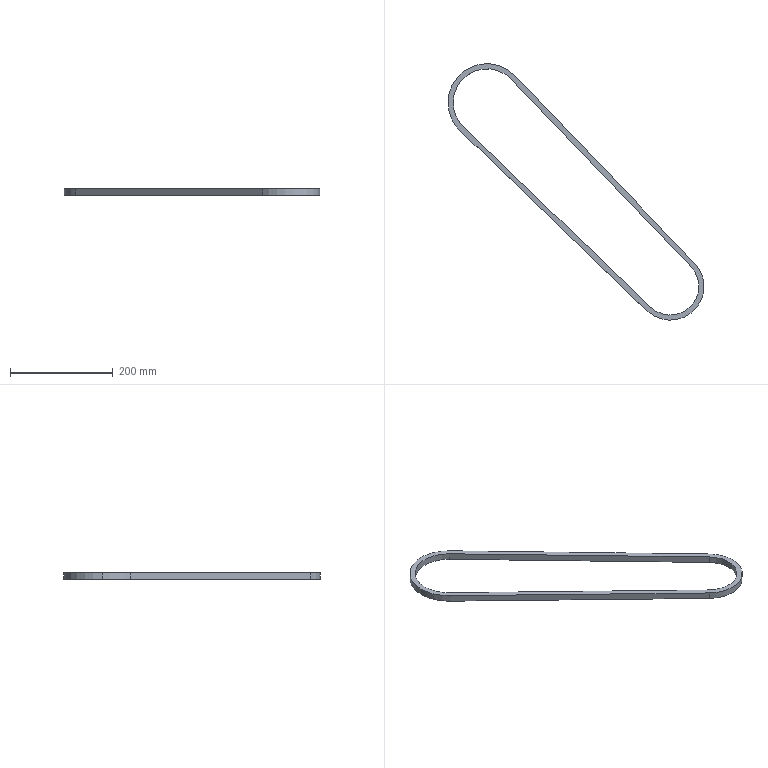Part | STEP file | Pasek_klinowy3V11 | 1 solid | 12 faces | box 497.285 x 498.317 x 13 mm | volume 184721 mm3 | cylinder 6 | plane 6 | commonest cylinder face diameters 131 x3 151 x2 111 x1
STEP:
#1=CARTESIAN_POINT('',(0.,0.,0.));
#2=DIRECTION('',(0.,0.,1.));
#3=DIRECTION('',(1.,0.,0.));
#4=AXIS2_PLACEMENT_3D('',#1,#2,#3);
#5=CARTESIAN_POINT('',(226.295,-74.498,13.));
#6=VERTEX_POINT('',#5);
#7=CARTESIAN_POINT('',(226.295,-74.498,0.));
#8=VERTEX_POINT('',#7);
#9=CARTESIAN_POINT('',(226.295,-74.498,13.));
#10=DIRECTION('',(0.,0.,-1.));
#11=VECTOR('',#10,1.);
#12=LINE('',#9,#11);
#13=CARTESIAN_POINT('',(179.005,-119.818,13.));
#14=DIRECTION('',(0.,0.,-1.));
#15=DIRECTION('',(-1.,0.,0.));
#16=AXIS2_PLACEMENT_3D('',#13,#14,#15);
#17=CYLINDRICAL_SURFACE('',#16,65.5);
#18=CARTESIAN_POINT('',(2.377,0.));
#19=DIRECTION('',(0.,1.));
#20=VECTOR('',#19,1.);
#21=LINE('',#18,#20);
#22=(GEOMETRIC_REPRESENTATION_CONTEXT(2)PARAMETRIC_REPRESENTATION_CONTEXT()REPRESENTATION_CONTEXT('',''));
#23=DEFINITIONAL_REPRESENTATION('',(#21),#22);
#24=PCURVE('',#17,#23);
#25=CARTESIAN_POINT('',(226.295,-74.498,13.));
#26=DIRECTION('',(-0.722,-0.6919,0.));
#27=DIRECTION('',(0.6919,-0.722,0.));
#28=AXIS2_PLACEMENT_3D('',#25,#26,#27);
#29=PLANE('',#28);
#30=CARTESIAN_POINT('',(0.,0.));
#31=DIRECTION('',(0.,-1.));
#32=VECTOR('',#31,1.);
#33=LINE('',#30,#32);
#34=(GEOMETRIC_REPRESENTATION_CONTEXT(2)PARAMETRIC_REPRESENTATION_CONTEXT()REPRESENTATION_CONTEXT('',''));
#35=DEFINITIONAL_REPRESENTATION('',(#33),#34);
#36=PCURVE('',#29,#35);
#37=SURFACE_CURVE('',#12,(#24,#36),.PCURVE_S1.);
#38=EDGE_CURVE('',#6,#8,#37,.T.);
#39=ORIENTED_EDGE('',*,*,#38,.T.);
#40=CARTESIAN_POINT('',(113.505,-119.818,0.));
#41=VERTEX_POINT('',#40);
#42=CARTESIAN_POINT('',(179.005,-119.818,0.));
#43=DIRECTION('',(0.,0.,1.));
#44=DIRECTION('',(1.,0.,0.));
#45=AXIS2_PLACEMENT_3D('',#42,#43,#44);
#46=CIRCLE('',#45,65.5);
#47=CARTESIAN_POINT('',(3.142,13.));
#48=DIRECTION('',(-1.,0.));
#49=VECTOR('',#48,1.);
#50=LINE('',#47,#49);
#51=(GEOMETRIC_REPRESENTATION_CONTEXT(2)PARAMETRIC_REPRESENTATION_CONTEXT()REPRESENTATION_CONTEXT('',''));
#52=DEFINITIONAL_REPRESENTATION('',(#50),#51);
#53=PCURVE('',#17,#52);
#54=CARTESIAN_POINT('',(179.005,-119.818,0.));
#55=DIRECTION('',(0.,0.,1.));
#56=DIRECTION('',(1.,0.,0.));
#57=AXIS2_PLACEMENT_3D('',#54,#55,#56);
#58=PLANE('',#57);
#59=CARTESIAN_POINT('',(0.,0.));
#60=DIRECTION('',(1.,0.));
#61=AXIS2_PLACEMENT_2D('',#59,#60);
#62=CIRCLE('',#61,65.5);
#63=(GEOMETRIC_REPRESENTATION_CONTEXT(2)PARAMETRIC_REPRESENTATION_CONTEXT()REPRESENTATION_CONTEXT('',''));
#64=DEFINITIONAL_REPRESENTATION('',(#62),#63);
#65=PCURVE('',#58,#64);
#66=SURFACE_CURVE('',#46,(#53,#65),.PCURVE_S1.);
#67=EDGE_CURVE('',#8,#41,#66,.T.);
#68=ORIENTED_EDGE('',*,*,#67,.T.);
#69=CARTESIAN_POINT('',(113.505,-119.818,13.));
#70=VERTEX_POINT('',#69);
#71=CARTESIAN_POINT('',(113.505,-119.818,13.));
#72=DIRECTION('',(0.,0.,-1.));
#73=VECTOR('',#72,1.);
#74=LINE('',#71,#73);
#75=CARTESIAN_POINT('',(0.,0.));
#76=DIRECTION('',(0.,1.));
#77=VECTOR('',#76,1.);
#78=LINE('',#75,#77);
#79=(GEOMETRIC_REPRESENTATION_CONTEXT(2)PARAMETRIC_REPRESENTATION_CONTEXT()REPRESENTATION_CONTEXT('',''));
#80=DEFINITIONAL_REPRESENTATION('',(#78),#79);
#81=PCURVE('',#17,#80);
#82=CARTESIAN_POINT('',(179.005,-119.818,13.));
#83=DIRECTION('',(0.,0.,-1.));
#84=DIRECTION('',(-1.,0.,0.));
#85=AXIS2_PLACEMENT_3D('',#82,#83,#84);
#86=CYLINDRICAL_SURFACE('',#85,65.5);
#87=CARTESIAN_POINT('',(6.283,0.));
#88=DIRECTION('',(0.,1.));
#89=VECTOR('',#88,1.);
#90=LINE('',#87,#89);
#91=(GEOMETRIC_REPRESENTATION_CONTEXT(2)PARAMETRIC_REPRESENTATION_CONTEXT()REPRESENTATION_CONTEXT('',''));
#92=DEFINITIONAL_REPRESENTATION('',(#90),#91);
#93=PCURVE('',#86,#92);
#94=SURFACE_CURVE('',#74,(#81,#93),.PCURVE_S1.);
#95=EDGE_CURVE('',#70,#41,#94,.T.);
#96=ORIENTED_EDGE('',*,*,#95,.F.);
#97=CARTESIAN_POINT('',(179.005,-119.818,13.));
#98=DIRECTION('',(0.,0.,1.));
#99=DIRECTION('',(1.,0.,0.));
#100=AXIS2_PLACEMENT_3D('',#97,#98,#99);
#101=CIRCLE('',#100,65.5);
#102=CARTESIAN_POINT('',(3.142,0.));
#103=DIRECTION('',(-1.,0.));
#104=VECTOR('',#103,1.);
#105=LINE('',#102,#104);
#106=(GEOMETRIC_REPRESENTATION_CONTEXT(2)PARAMETRIC_REPRESENTATION_CONTEXT()REPRESENTATION_CONTEXT('',''));
#107=DEFINITIONAL_REPRESENTATION('',(#105),#106);
#108=PCURVE('',#17,#107);
#109=CARTESIAN_POINT('',(179.005,-119.818,13.));
#110=DIRECTION('',(0.,0.,1.));
#111=DIRECTION('',(1.,0.,0.));
#112=AXIS2_PLACEMENT_3D('',#109,#110,#111);
#113=PLANE('',#112);
#114=CARTESIAN_POINT('',(0.,0.));
#115=DIRECTION('',(1.,0.));
#116=AXIS2_PLACEMENT_2D('',#114,#115);
#117=CIRCLE('',#116,65.5);
#118=(GEOMETRIC_REPRESENTATION_CONTEXT(2)PARAMETRIC_REPRESENTATION_CONTEXT()REPRESENTATION_CONTEXT('',''));
#119=DEFINITIONAL_REPRESENTATION('',(#117),#118);
#120=PCURVE('',#113,#119);
#121=SURFACE_CURVE('',#101,(#108,#120),.PCURVE_S1.);
#122=EDGE_CURVE('',#6,#70,#121,.T.);
#123=ORIENTED_EDGE('',*,*,#122,.F.);
#124=EDGE_LOOP('',(#39,#68,#96,#123));
#125=FACE_BOUND('',#124,.F.);
#126=ADVANCED_FACE('',(#125),#17,.F.);
#127=CARTESIAN_POINT('',(103.505,-119.818,13.));
#128=VERTEX_POINT('',#127);
#129=CARTESIAN_POINT('',(126.608,-174.177,13.));
#130=VERTEX_POINT('',#129);
#131=CARTESIAN_POINT('',(179.005,-119.818,13.));
#132=DIRECTION('',(0.,0.,1.));
#133=DIRECTION('',(1.,0.,0.));
#134=AXIS2_PLACEMENT_3D('',#131,#132,#133);
#135=CIRCLE('',#134,75.5);
#136=CARTESIAN_POINT('',(179.005,-119.818,13.));
#137=DIRECTION('',(0.,0.,-1.));
#138=DIRECTION('',(-1.,0.,0.));
#139=AXIS2_PLACEMENT_3D('',#136,#137,#138);
#140=CYLINDRICAL_SURFACE('',#139,75.5);
#141=CARTESIAN_POINT('',(9.425,0.));
#142=DIRECTION('',(-1.,0.));
#143=VECTOR('',#142,1.);
#144=LINE('',#141,#143);
#145=(GEOMETRIC_REPRESENTATION_CONTEXT(2)PARAMETRIC_REPRESENTATION_CONTEXT()REPRESENTATION_CONTEXT('',''));
#146=DEFINITIONAL_REPRESENTATION('',(#144),#145);
#147=PCURVE('',#140,#146);
#148=CARTESIAN_POINT('',(0.,0.));
#149=DIRECTION('',(1.,0.));
#150=AXIS2_PLACEMENT_2D('',#148,#149);
#151=CIRCLE('',#150,75.5);
#152=(GEOMETRIC_REPRESENTATION_CONTEXT(2)PARAMETRIC_REPRESENTATION_CONTEXT()REPRESENTATION_CONTEXT('',''));
#153=DEFINITIONAL_REPRESENTATION('',(#151),#152);
#154=PCURVE('',#113,#153);
#155=SURFACE_CURVE('',#135,(#147,#154),.PCURVE_S1.);
#156=EDGE_CURVE('',#128,#130,#155,.T.);
#157=ORIENTED_EDGE('',*,*,#156,.F.);
#158=CARTESIAN_POINT('',(103.505,-119.818,0.));
#159=VERTEX_POINT('',#158);
#160=CARTESIAN_POINT('',(103.505,-119.818,13.));
#161=DIRECTION('',(0.,0.,-1.));
#162=VECTOR('',#161,1.);
#163=LINE('',#160,#162);
#164=CARTESIAN_POINT('',(6.283,0.));
#165=DIRECTION('',(0.,1.));
#166=VECTOR('',#165,1.);
#167=LINE('',#164,#166);
#168=(GEOMETRIC_REPRESENTATION_CONTEXT(2)PARAMETRIC_REPRESENTATION_CONTEXT()REPRESENTATION_CONTEXT('',''));
#169=DEFINITIONAL_REPRESENTATION('',(#167),#168);
#170=PCURVE('',#140,#169);
#171=CARTESIAN_POINT('',(179.005,-119.818,13.));
#172=DIRECTION('',(0.,0.,-1.));
#173=DIRECTION('',(-1.,0.,0.));
#174=AXIS2_PLACEMENT_3D('',#171,#172,#173);
#175=CYLINDRICAL_SURFACE('',#174,75.5);
#176=CARTESIAN_POINT('',(0.,0.));
#177=DIRECTION('',(0.,1.));
#178=VECTOR('',#177,1.);
#179=LINE('',#176,#178);
#180=(GEOMETRIC_REPRESENTATION_CONTEXT(2)PARAMETRIC_REPRESENTATION_CONTEXT()REPRESENTATION_CONTEXT('',''));
#181=DEFINITIONAL_REPRESENTATION('',(#179),#180);
#182=PCURVE('',#175,#181);
#183=SURFACE_CURVE('',#163,(#170,#182),.PCURVE_S1.);
#184=EDGE_CURVE('',#128,#159,#183,.T.);
#185=ORIENTED_EDGE('',*,*,#184,.T.);
#186=CARTESIAN_POINT('',(126.608,-174.177,0.));
#187=VERTEX_POINT('',#186);
#188=CARTESIAN_POINT('',(179.005,-119.818,0.));
#189=DIRECTION('',(0.,0.,1.));
#190=DIRECTION('',(1.,0.,0.));
#191=AXIS2_PLACEMENT_3D('',#188,#189,#190);
#192=CIRCLE('',#191,75.5);
#193=CARTESIAN_POINT('',(9.425,13.));
#194=DIRECTION('',(-1.,0.));
#195=VECTOR('',#194,1.);
#196=LINE('',#193,#195);
#197=(GEOMETRIC_REPRESENTATION_CONTEXT(2)PARAMETRIC_REPRESENTATION_CONTEXT()REPRESENTATION_CONTEXT('',''));
#198=DEFINITIONAL_REPRESENTATION('',(#196),#197);
#199=PCURVE('',#140,#198);
#200=CARTESIAN_POINT('',(0.,0.));
#201=DIRECTION('',(1.,0.));
#202=AXIS2_PLACEMENT_2D('',#200,#201);
#203=CIRCLE('',#202,75.5);
#204=(GEOMETRIC_REPRESENTATION_CONTEXT(2)PARAMETRIC_REPRESENTATION_CONTEXT()REPRESENTATION_CONTEXT('',''));
#205=DEFINITIONAL_REPRESENTATION('',(#203),#204);
#206=PCURVE('',#58,#205);
#207=SURFACE_CURVE('',#192,(#199,#206),.PCURVE_S1.);
#208=EDGE_CURVE('',#159,#187,#207,.T.);
#209=ORIENTED_EDGE('',*,*,#208,.T.);
#210=CARTESIAN_POINT('',(126.608,-174.177,13.));
#211=DIRECTION('',(0.,0.,-1.));
#212=VECTOR('',#211,1.);
#213=LINE('',#210,#212);
#214=CARTESIAN_POINT('',(5.479,0.));
#215=DIRECTION('',(0.,1.));
#216=VECTOR('',#215,1.);
#217=LINE('',#214,#216);
#218=(GEOMETRIC_REPRESENTATION_CONTEXT(2)PARAMETRIC_REPRESENTATION_CONTEXT()REPRESENTATION_CONTEXT('',''));
#219=DEFINITIONAL_REPRESENTATION('',(#217),#218);
#220=PCURVE('',#140,#219);
#221=CARTESIAN_POINT('',(126.608,-174.177,13.));
#222=DIRECTION('',(0.694,0.72,0.));
#223=DIRECTION('',(-0.72,0.694,0.));
#224=AXIS2_PLACEMENT_3D('',#221,#222,#223);
#225=PLANE('',#224);
#226=CARTESIAN_POINT('',(0.,0.));
#227=DIRECTION('',(0.,-1.));
#228=VECTOR('',#227,1.);
#229=LINE('',#226,#228);
#230=(GEOMETRIC_REPRESENTATION_CONTEXT(2)PARAMETRIC_REPRESENTATION_CONTEXT()REPRESENTATION_CONTEXT('',''));
#231=DEFINITIONAL_REPRESENTATION('',(#229),#230);
#232=PCURVE('',#225,#231);
#233=SURFACE_CURVE('',#213,(#220,#232),.PCURVE_S1.);
#234=EDGE_CURVE('',#130,#187,#233,.T.);
#235=ORIENTED_EDGE('',*,*,#234,.F.);
#236=EDGE_LOOP('',(#157,#185,#209,#235));
#237=FACE_BOUND('',#236,.T.);
#238=ADVANCED_FACE('',(#237),#140,.T.);
#239=CARTESIAN_POINT('',(233.515,-67.579,13.));
#240=VERTEX_POINT('',#239);
#241=CARTESIAN_POINT('',(179.005,-119.818,13.));
#242=DIRECTION('',(0.,0.,1.));
#243=DIRECTION('',(1.,0.,0.));
#244=AXIS2_PLACEMENT_3D('',#241,#242,#243);
#245=CIRCLE('',#244,75.5);
#246=CARTESIAN_POINT('',(0.,0.));
#247=DIRECTION('',(1.,0.));
#248=AXIS2_PLACEMENT_2D('',#246,#247);
#249=CIRCLE('',#248,75.5);
#250=(GEOMETRIC_REPRESENTATION_CONTEXT(2)PARAMETRIC_REPRESENTATION_CONTEXT()REPRESENTATION_CONTEXT('',''));
#251=DEFINITIONAL_REPRESENTATION('',(#249),#250);
#252=PCURVE('',#113,#251);
#253=CARTESIAN_POINT('',(3.142,0.));
#254=DIRECTION('',(-1.,0.));
#255=VECTOR('',#254,1.);
#256=LINE('',#253,#255);
#257=(GEOMETRIC_REPRESENTATION_CONTEXT(2)PARAMETRIC_REPRESENTATION_CONTEXT()REPRESENTATION_CONTEXT('',''));
#258=DEFINITIONAL_REPRESENTATION('',(#256),#257);
#259=PCURVE('',#175,#258);
#260=SURFACE_CURVE('',#245,(#252,#259),.PCURVE_S1.);
#261=EDGE_CURVE('',#240,#128,#260,.T.);
#262=ORIENTED_EDGE('',*,*,#261,.T.);
#263=ORIENTED_EDGE('',*,*,#156,.T.);
#264=CARTESIAN_POINT('',(489.833,-524.293,13.));
#265=VERTEX_POINT('',#264);
#266=CARTESIAN_POINT('',(126.608,-174.177,13.));
#267=DIRECTION('',(0.72,-0.694,0.));
#268=VECTOR('',#267,1.);
#269=LINE('',#266,#268);
#270=CARTESIAN_POINT('',(-52.397,-54.358));
#271=DIRECTION('',(0.72,-0.694));
#272=VECTOR('',#271,1.);
#273=LINE('',#270,#272);
#274=(GEOMETRIC_REPRESENTATION_CONTEXT(2)PARAMETRIC_REPRESENTATION_CONTEXT()REPRESENTATION_CONTEXT('',''));
#275=DEFINITIONAL_REPRESENTATION('',(#273),#274);
#276=PCURVE('',#113,#275);
#277=CARTESIAN_POINT('',(0.,0.));
#278=DIRECTION('',(-1.,0.));
#279=VECTOR('',#278,1.);
#280=LINE('',#277,#279);
#281=(GEOMETRIC_REPRESENTATION_CONTEXT(2)PARAMETRIC_REPRESENTATION_CONTEXT()REPRESENTATION_CONTEXT('',''));
#282=DEFINITIONAL_REPRESENTATION('',(#280),#281);
#283=PCURVE('',#225,#282);
#284=SURFACE_CURVE('',#269,(#276,#283),.PCURVE_S1.);
#285=EDGE_CURVE('',#130,#265,#284,.T.);
#286=ORIENTED_EDGE('',*,*,#285,.T.);
#287=CARTESIAN_POINT('',(582.58,-431.815,13.));
#288=VERTEX_POINT('',#287);
#289=CARTESIAN_POINT('',(535.29,-477.135,13.));
#290=DIRECTION('',(0.,0.,1.));
#291=DIRECTION('',(1.,0.,0.));
#292=AXIS2_PLACEMENT_3D('',#289,#290,#291);
#293=CIRCLE('',#292,65.5);
#294=CARTESIAN_POINT('',(356.285,-357.317));
#295=DIRECTION('',(1.,0.));
#296=AXIS2_PLACEMENT_2D('',#294,#295);
#297=CIRCLE('',#296,65.5);
#298=(GEOMETRIC_REPRESENTATION_CONTEXT(2)PARAMETRIC_REPRESENTATION_CONTEXT()REPRESENTATION_CONTEXT('',''));
#299=DEFINITIONAL_REPRESENTATION('',(#297),#298);
#300=PCURVE('',#113,#299);
#301=CARTESIAN_POINT('',(535.29,-477.135,13.));
#302=DIRECTION('',(0.,0.,-1.));
#303=DIRECTION('',(-1.,0.,0.));
#304=AXIS2_PLACEMENT_3D('',#301,#302,#303);
#305=CYLINDRICAL_SURFACE('',#304,65.5);
#306=CARTESIAN_POINT('',(9.425,0.));
#307=DIRECTION('',(-1.,0.));
#308=VECTOR('',#307,1.);
#309=LINE('',#306,#308);
#310=(GEOMETRIC_REPRESENTATION_CONTEXT(2)PARAMETRIC_REPRESENTATION_CONTEXT()REPRESENTATION_CONTEXT('',''));
#311=DEFINITIONAL_REPRESENTATION('',(#309),#310);
#312=PCURVE('',#305,#311);
#313=SURFACE_CURVE('',#293,(#300,#312),.PCURVE_S1.);
#314=EDGE_CURVE('',#265,#288,#313,.T.);
#315=ORIENTED_EDGE('',*,*,#314,.T.);
#316=CARTESIAN_POINT('',(233.515,-67.579,13.));
#317=DIRECTION('',(-0.6919,0.722,0.));
#318=VECTOR('',#317,1.);
#319=LINE('',#316,#318);
#320=CARTESIAN_POINT('',(54.51,52.239));
#321=DIRECTION('',(-0.6919,0.722));
#322=VECTOR('',#321,1.);
#323=LINE('',#320,#322);
#324=(GEOMETRIC_REPRESENTATION_CONTEXT(2)PARAMETRIC_REPRESENTATION_CONTEXT()REPRESENTATION_CONTEXT('',''));
#325=DEFINITIONAL_REPRESENTATION('',(#323),#324);
#326=PCURVE('',#113,#325);
#327=CARTESIAN_POINT('',(233.515,-67.579,13.));
#328=DIRECTION('',(-0.722,-0.6919,0.));
#329=DIRECTION('',(0.6919,-0.722,0.));
#330=AXIS2_PLACEMENT_3D('',#327,#328,#329);
#331=PLANE('',#330);
#332=CARTESIAN_POINT('',(0.,0.));
#333=DIRECTION('',(-1.,0.));
#334=VECTOR('',#333,1.);
#335=LINE('',#332,#334);
#336=(GEOMETRIC_REPRESENTATION_CONTEXT(2)PARAMETRIC_REPRESENTATION_CONTEXT()REPRESENTATION_CONTEXT('',''));
#337=DEFINITIONAL_REPRESENTATION('',(#335),#336);
#338=PCURVE('',#331,#337);
#339=SURFACE_CURVE('',#319,(#326,#338),.PCURVE_S1.);
#340=EDGE_CURVE('',#288,#240,#339,.T.);
#341=ORIENTED_EDGE('',*,*,#340,.T.);
#342=EDGE_LOOP('',(#262,#263,#286,#315,#341));
#343=FACE_BOUND('',#342,.T.);
#344=CARTESIAN_POINT('',(133.548,-166.977,13.));
#345=VERTEX_POINT('',#344);
#346=CARTESIAN_POINT('',(496.773,-517.094,13.));
#347=VERTEX_POINT('',#346);
#348=CARTESIAN_POINT('',(133.548,-166.977,13.));
#349=DIRECTION('',(0.72,-0.694,0.));
#350=VECTOR('',#349,1.);
#351=LINE('',#348,#350);
#352=CARTESIAN_POINT('',(-45.457,-47.159));
#353=DIRECTION('',(0.72,-0.694));
#354=VECTOR('',#353,1.);
#355=LINE('',#352,#354);
#356=(GEOMETRIC_REPRESENTATION_CONTEXT(2)PARAMETRIC_REPRESENTATION_CONTEXT()REPRESENTATION_CONTEXT('',''));
#357=DEFINITIONAL_REPRESENTATION('',(#355),#356);
#358=PCURVE('',#113,#357);
#359=CARTESIAN_POINT('',(133.548,-166.977,13.));
#360=DIRECTION('',(0.694,0.72,0.));
#361=DIRECTION('',(-0.72,0.694,0.));
#362=AXIS2_PLACEMENT_3D('',#359,#360,#361);
#363=PLANE('',#362);
#364=CARTESIAN_POINT('',(0.,0.));
#365=DIRECTION('',(-1.,0.));
#366=VECTOR('',#365,1.);
#367=LINE('',#364,#366);
#368=(GEOMETRIC_REPRESENTATION_CONTEXT(2)PARAMETRIC_REPRESENTATION_CONTEXT()REPRESENTATION_CONTEXT('',''));
#369=DEFINITIONAL_REPRESENTATION('',(#367),#368);
#370=PCURVE('',#363,#369);
#371=SURFACE_CURVE('',#351,(#358,#370),.PCURVE_S1.);
#372=EDGE_CURVE('',#345,#347,#371,.T.);
#373=ORIENTED_EDGE('',*,*,#372,.F.);
#374=CARTESIAN_POINT('',(179.005,-119.818,13.));
#375=DIRECTION('',(0.,0.,1.));
#376=DIRECTION('',(1.,0.,0.));
#377=AXIS2_PLACEMENT_3D('',#374,#375,#376);
#378=CIRCLE('',#377,65.5);
#379=CARTESIAN_POINT('',(0.,0.));
#380=DIRECTION('',(1.,0.));
#381=AXIS2_PLACEMENT_2D('',#379,#380);
#382=CIRCLE('',#381,65.5);
#383=(GEOMETRIC_REPRESENTATION_CONTEXT(2)PARAMETRIC_REPRESENTATION_CONTEXT()REPRESENTATION_CONTEXT('',''));
#384=DEFINITIONAL_REPRESENTATION('',(#382),#383);
#385=PCURVE('',#113,#384);
#386=CARTESIAN_POINT('',(9.425,0.));
#387=DIRECTION('',(-1.,0.));
#388=VECTOR('',#387,1.);
#389=LINE('',#386,#388);
#390=(GEOMETRIC_REPRESENTATION_CONTEXT(2)PARAMETRIC_REPRESENTATION_CONTEXT()REPRESENTATION_CONTEXT('',''));
#391=DEFINITIONAL_REPRESENTATION('',(#389),#390);
#392=PCURVE('',#86,#391);
#393=SURFACE_CURVE('',#378,(#385,#392),.PCURVE_S1.);
#394=EDGE_CURVE('',#70,#345,#393,.T.);
#395=ORIENTED_EDGE('',*,*,#394,.F.);
#396=ORIENTED_EDGE('',*,*,#122,.F.);
#397=CARTESIAN_POINT('',(575.36,-438.734,13.));
#398=VERTEX_POINT('',#397);
#399=CARTESIAN_POINT('',(226.295,-74.498,13.));
#400=DIRECTION('',(-0.6919,0.722,0.));
#401=VECTOR('',#400,1.);
#402=LINE('',#399,#401);
#403=CARTESIAN_POINT('',(47.29,45.32));
#404=DIRECTION('',(-0.6919,0.722));
#405=VECTOR('',#404,1.);
#406=LINE('',#403,#405);
#407=(GEOMETRIC_REPRESENTATION_CONTEXT(2)PARAMETRIC_REPRESENTATION_CONTEXT()REPRESENTATION_CONTEXT('',''));
#408=DEFINITIONAL_REPRESENTATION('',(#406),#407);
#409=PCURVE('',#113,#408);
#410=CARTESIAN_POINT('',(0.,0.));
#411=DIRECTION('',(-1.,0.));
#412=VECTOR('',#411,1.);
#413=LINE('',#410,#412);
#414=(GEOMETRIC_REPRESENTATION_CONTEXT(2)PARAMETRIC_REPRESENTATION_CONTEXT()REPRESENTATION_CONTEXT('',''));
#415=DEFINITIONAL_REPRESENTATION('',(#413),#414);
#416=PCURVE('',#29,#415);
#417=SURFACE_CURVE('',#402,(#409,#416),.PCURVE_S1.);
#418=EDGE_CURVE('',#398,#6,#417,.T.);
#419=ORIENTED_EDGE('',*,*,#418,.F.);
#420=CARTESIAN_POINT('',(535.29,-477.135,13.));
#421=DIRECTION('',(0.,0.,1.));
#422=DIRECTION('',(1.,0.,0.));
#423=AXIS2_PLACEMENT_3D('',#420,#421,#422);
#424=CIRCLE('',#423,55.5);
#425=CARTESIAN_POINT('',(356.285,-357.317));
#426=DIRECTION('',(1.,0.));
#427=AXIS2_PLACEMENT_2D('',#425,#426);
#428=CIRCLE('',#427,55.5);
#429=(GEOMETRIC_REPRESENTATION_CONTEXT(2)PARAMETRIC_REPRESENTATION_CONTEXT()REPRESENTATION_CONTEXT('',''));
#430=DEFINITIONAL_REPRESENTATION('',(#428),#429);
#431=PCURVE('',#113,#430);
#432=CARTESIAN_POINT('',(535.29,-477.135,13.));
#433=DIRECTION('',(0.,0.,-1.));
#434=DIRECTION('',(-1.,0.,0.));
#435=AXIS2_PLACEMENT_3D('',#432,#433,#434);
#436=CYLINDRICAL_SURFACE('',#435,55.5);
#437=CARTESIAN_POINT('',(9.425,0.));
#438=DIRECTION('',(-1.,0.));
#439=VECTOR('',#438,1.);
#440=LINE('',#437,#439);
#441=(GEOMETRIC_REPRESENTATION_CONTEXT(2)PARAMETRIC_REPRESENTATION_CONTEXT()REPRESENTATION_CONTEXT('',''));
#442=DEFINITIONAL_REPRESENTATION('',(#440),#441);
#443=PCURVE('',#436,#442);
#444=SURFACE_CURVE('',#424,(#431,#443),.PCURVE_S1.);
#445=EDGE_CURVE('',#347,#398,#444,.T.);
#446=ORIENTED_EDGE('',*,*,#445,.F.);
#447=EDGE_LOOP('',(#373,#395,#396,#419,#446));
#448=FACE_BOUND('',#447,.T.);
#449=ADVANCED_FACE('',(#343,#448),#113,.T.);
#450=CARTESIAN_POINT('',(233.515,-67.579,0.));
#451=VERTEX_POINT('',#450);
#452=CARTESIAN_POINT('',(179.005,-119.818,0.));
#453=DIRECTION('',(0.,0.,1.));
#454=DIRECTION('',(1.,0.,0.));
#455=AXIS2_PLACEMENT_3D('',#452,#453,#454);
#456=CIRCLE('',#455,75.5);
#457=CARTESIAN_POINT('',(0.,0.));
#458=DIRECTION('',(1.,0.));
#459=AXIS2_PLACEMENT_2D('',#457,#458);
#460=CIRCLE('',#459,75.5);
#461=(GEOMETRIC_REPRESENTATION_CONTEXT(2)PARAMETRIC_REPRESENTATION_CONTEXT()REPRESENTATION_CONTEXT('',''));
#462=DEFINITIONAL_REPRESENTATION('',(#460),#461);
#463=PCURVE('',#58,#462);
#464=CARTESIAN_POINT('',(3.142,13.));
#465=DIRECTION('',(-1.,0.));
#466=VECTOR('',#465,1.);
#467=LINE('',#464,#466);
#468=(GEOMETRIC_REPRESENTATION_CONTEXT(2)PARAMETRIC_REPRESENTATION_CONTEXT()REPRESENTATION_CONTEXT('',''));
#469=DEFINITIONAL_REPRESENTATION('',(#467),#468);
#470=PCURVE('',#175,#469);
#471=SURFACE_CURVE('',#456,(#463,#470),.PCURVE_S1.);
#472=EDGE_CURVE('',#451,#159,#471,.T.);
#473=ORIENTED_EDGE('',*,*,#472,.F.);
#474=CARTESIAN_POINT('',(582.58,-431.815,0.));
#475=VERTEX_POINT('',#474);
#476=CARTESIAN_POINT('',(233.515,-67.579,0.));
#477=DIRECTION('',(-0.6919,0.722,0.));
#478=VECTOR('',#477,1.);
#479=LINE('',#476,#478);
#480=CARTESIAN_POINT('',(54.51,52.239));
#481=DIRECTION('',(-0.6919,0.722));
#482=VECTOR('',#481,1.);
#483=LINE('',#480,#482);
#484=(GEOMETRIC_REPRESENTATION_CONTEXT(2)PARAMETRIC_REPRESENTATION_CONTEXT()REPRESENTATION_CONTEXT('',''));
#485=DEFINITIONAL_REPRESENTATION('',(#483),#484);
#486=PCURVE('',#58,#485);
#487=CARTESIAN_POINT('',(0.,-13.));
#488=DIRECTION('',(-1.,0.));
#489=VECTOR('',#488,1.);
#490=LINE('',#487,#489);
#491=(GEOMETRIC_REPRESENTATION_CONTEXT(2)PARAMETRIC_REPRESENTATION_CONTEXT()REPRESENTATION_CONTEXT('',''));
#492=DEFINITIONAL_REPRESENTATION('',(#490),#491);
#493=PCURVE('',#331,#492);
#494=SURFACE_CURVE('',#479,(#486,#493),.PCURVE_S1.);
#495=EDGE_CURVE('',#475,#451,#494,.T.);
#496=ORIENTED_EDGE('',*,*,#495,.F.);
#497=CARTESIAN_POINT('',(489.833,-524.293,0.));
#498=VERTEX_POINT('',#497);
#499=CARTESIAN_POINT('',(535.29,-477.135,0.));
#500=DIRECTION('',(0.,0.,1.));
#501=DIRECTION('',(1.,0.,0.));
#502=AXIS2_PLACEMENT_3D('',#499,#500,#501);
#503=CIRCLE('',#502,65.5);
#504=CARTESIAN_POINT('',(356.285,-357.317));
#505=DIRECTION('',(1.,0.));
#506=AXIS2_PLACEMENT_2D('',#504,#505);
#507=CIRCLE('',#506,65.5);
#508=(GEOMETRIC_REPRESENTATION_CONTEXT(2)PARAMETRIC_REPRESENTATION_CONTEXT()REPRESENTATION_CONTEXT('',''));
#509=DEFINITIONAL_REPRESENTATION('',(#507),#508);
#510=PCURVE('',#58,#509);
#511=CARTESIAN_POINT('',(9.425,13.));
#512=DIRECTION('',(-1.,0.));
#513=VECTOR('',#512,1.);
#514=LINE('',#511,#513);
#515=(GEOMETRIC_REPRESENTATION_CONTEXT(2)PARAMETRIC_REPRESENTATION_CONTEXT()REPRESENTATION_CONTEXT('',''));
#516=DEFINITIONAL_REPRESENTATION('',(#514),#515);
#517=PCURVE('',#305,#516);
#518=SURFACE_CURVE('',#503,(#510,#517),.PCURVE_S1.);
#519=EDGE_CURVE('',#498,#475,#518,.T.);
#520=ORIENTED_EDGE('',*,*,#519,.F.);
#521=CARTESIAN_POINT('',(126.608,-174.177,0.));
#522=DIRECTION('',(0.72,-0.694,0.));
#523=VECTOR('',#522,1.);
#524=LINE('',#521,#523);
#525=CARTESIAN_POINT('',(-52.397,-54.358));
#526=DIRECTION('',(0.72,-0.694));
#527=VECTOR('',#526,1.);
#528=LINE('',#525,#527);
#529=(GEOMETRIC_REPRESENTATION_CONTEXT(2)PARAMETRIC_REPRESENTATION_CONTEXT()REPRESENTATION_CONTEXT('',''));
#530=DEFINITIONAL_REPRESENTATION('',(#528),#529);
#531=PCURVE('',#58,#530);
#532=CARTESIAN_POINT('',(0.,-13.));
#533=DIRECTION('',(-1.,0.));
#534=VECTOR('',#533,1.);
#535=LINE('',#532,#534);
#536=(GEOMETRIC_REPRESENTATION_CONTEXT(2)PARAMETRIC_REPRESENTATION_CONTEXT()REPRESENTATION_CONTEXT('',''));
#537=DEFINITIONAL_REPRESENTATION('',(#535),#536);
#538=PCURVE('',#225,#537);
#539=SURFACE_CURVE('',#524,(#531,#538),.PCURVE_S1.);
#540=EDGE_CURVE('',#187,#498,#539,.T.);
#541=ORIENTED_EDGE('',*,*,#540,.F.);
#542=ORIENTED_EDGE('',*,*,#208,.F.);
#543=EDGE_LOOP('',(#473,#496,#520,#541,#542));
#544=FACE_BOUND('',#543,.T.);
#545=ORIENTED_EDGE('',*,*,#67,.T.);
#546=CARTESIAN_POINT('',(133.548,-166.977,0.));
#547=VERTEX_POINT('',#546);
#548=CARTESIAN_POINT('',(179.005,-119.818,0.));
#549=DIRECTION('',(0.,0.,1.));
#550=DIRECTION('',(1.,0.,0.));
#551=AXIS2_PLACEMENT_3D('',#548,#549,#550);
#552=CIRCLE('',#551,65.5);
#553=CARTESIAN_POINT('',(0.,0.));
#554=DIRECTION('',(1.,0.));
#555=AXIS2_PLACEMENT_2D('',#553,#554);
#556=CIRCLE('',#555,65.5);
#557=(GEOMETRIC_REPRESENTATION_CONTEXT(2)PARAMETRIC_REPRESENTATION_CONTEXT()REPRESENTATION_CONTEXT('',''));
#558=DEFINITIONAL_REPRESENTATION('',(#556),#557);
#559=PCURVE('',#58,#558);
#560=CARTESIAN_POINT('',(9.425,13.));
#561=DIRECTION('',(-1.,0.));
#562=VECTOR('',#561,1.);
#563=LINE('',#560,#562);
#564=(GEOMETRIC_REPRESENTATION_CONTEXT(2)PARAMETRIC_REPRESENTATION_CONTEXT()REPRESENTATION_CONTEXT('',''));
#565=DEFINITIONAL_REPRESENTATION('',(#563),#564);
#566=PCURVE('',#86,#565);
#567=SURFACE_CURVE('',#552,(#559,#566),.PCURVE_S1.);
#568=EDGE_CURVE('',#41,#547,#567,.T.);
#569=ORIENTED_EDGE('',*,*,#568,.T.);
#570=CARTESIAN_POINT('',(496.773,-517.094,0.));
#571=VERTEX_POINT('',#570);
#572=CARTESIAN_POINT('',(133.548,-166.977,0.));
#573=DIRECTION('',(0.72,-0.694,0.));
#574=VECTOR('',#573,1.);
#575=LINE('',#572,#574);
#576=CARTESIAN_POINT('',(-45.457,-47.159));
#577=DIRECTION('',(0.72,-0.694));
#578=VECTOR('',#577,1.);
#579=LINE('',#576,#578);
#580=(GEOMETRIC_REPRESENTATION_CONTEXT(2)PARAMETRIC_REPRESENTATION_CONTEXT()REPRESENTATION_CONTEXT('',''));
#581=DEFINITIONAL_REPRESENTATION('',(#579),#580);
#582=PCURVE('',#58,#581);
#583=CARTESIAN_POINT('',(0.,-13.));
#584=DIRECTION('',(-1.,0.));
#585=VECTOR('',#584,1.);
#586=LINE('',#583,#585);
#587=(GEOMETRIC_REPRESENTATION_CONTEXT(2)PARAMETRIC_REPRESENTATION_CONTEXT()REPRESENTATION_CONTEXT('',''));
#588=DEFINITIONAL_REPRESENTATION('',(#586),#587);
#589=PCURVE('',#363,#588);
#590=SURFACE_CURVE('',#575,(#582,#589),.PCURVE_S1.);
#591=EDGE_CURVE('',#547,#571,#590,.T.);
#592=ORIENTED_EDGE('',*,*,#591,.T.);
#593=CARTESIAN_POINT('',(575.36,-438.734,0.));
#594=VERTEX_POINT('',#593);
#595=CARTESIAN_POINT('',(535.29,-477.135,0.));
#596=DIRECTION('',(0.,0.,1.));
#597=DIRECTION('',(1.,0.,0.));
#598=AXIS2_PLACEMENT_3D('',#595,#596,#597);
#599=CIRCLE('',#598,55.5);
#600=CARTESIAN_POINT('',(356.285,-357.317));
#601=DIRECTION('',(1.,0.));
#602=AXIS2_PLACEMENT_2D('',#600,#601);
#603=CIRCLE('',#602,55.5);
#604=(GEOMETRIC_REPRESENTATION_CONTEXT(2)PARAMETRIC_REPRESENTATION_CONTEXT()REPRESENTATION_CONTEXT('',''));
#605=DEFINITIONAL_REPRESENTATION('',(#603),#604);
#606=PCURVE('',#58,#605);
#607=CARTESIAN_POINT('',(9.425,13.));
#608=DIRECTION('',(-1.,0.));
#609=VECTOR('',#608,1.);
#610=LINE('',#607,#609);
#611=(GEOMETRIC_REPRESENTATION_CONTEXT(2)PARAMETRIC_REPRESENTATION_CONTEXT()REPRESENTATION_CONTEXT('',''));
#612=DEFINITIONAL_REPRESENTATION('',(#610),#611);
#613=PCURVE('',#436,#612);
#614=SURFACE_CURVE('',#599,(#606,#613),.PCURVE_S1.);
#615=EDGE_CURVE('',#571,#594,#614,.T.);
#616=ORIENTED_EDGE('',*,*,#615,.T.);
#617=CARTESIAN_POINT('',(226.295,-74.498,0.));
#618=DIRECTION('',(-0.6919,0.722,0.));
#619=VECTOR('',#618,1.);
#620=LINE('',#617,#619);
#621=CARTESIAN_POINT('',(47.29,45.32));
#622=DIRECTION('',(-0.6919,0.722));
#623=VECTOR('',#622,1.);
#624=LINE('',#621,#623);
#625=(GEOMETRIC_REPRESENTATION_CONTEXT(2)PARAMETRIC_REPRESENTATION_CONTEXT()REPRESENTATION_CONTEXT('',''));
#626=DEFINITIONAL_REPRESENTATION('',(#624),#625);
#627=PCURVE('',#58,#626);
#628=CARTESIAN_POINT('',(0.,-13.));
#629=DIRECTION('',(-1.,0.));
#630=VECTOR('',#629,1.);
#631=LINE('',#628,#630);
#632=(GEOMETRIC_REPRESENTATION_CONTEXT(2)PARAMETRIC_REPRESENTATION_CONTEXT()REPRESENTATION_CONTEXT('',''));
#633=DEFINITIONAL_REPRESENTATION('',(#631),#632);
#634=PCURVE('',#29,#633);
#635=SURFACE_CURVE('',#620,(#627,#634),.PCURVE_S1.);
#636=EDGE_CURVE('',#594,#8,#635,.T.);
#637=ORIENTED_EDGE('',*,*,#636,.T.);
#638=EDGE_LOOP('',(#545,#569,#592,#616,#637));
#639=FACE_BOUND('',#638,.T.);
#640=ADVANCED_FACE('',(#544,#639),#58,.F.);
#641=ORIENTED_EDGE('',*,*,#184,.F.);
#642=ORIENTED_EDGE('',*,*,#261,.F.);
#643=CARTESIAN_POINT('',(233.515,-67.579,13.));
#644=DIRECTION('',(0.,0.,-1.));
#645=VECTOR('',#644,1.);
#646=LINE('',#643,#645);
#647=CARTESIAN_POINT('',(2.377,0.));
#648=DIRECTION('',(0.,1.));
#649=VECTOR('',#648,1.);
#650=LINE('',#647,#649);
#651=(GEOMETRIC_REPRESENTATION_CONTEXT(2)PARAMETRIC_REPRESENTATION_CONTEXT()REPRESENTATION_CONTEXT('',''));
#652=DEFINITIONAL_REPRESENTATION('',(#650),#651);
#653=PCURVE('',#175,#652);
#654=CARTESIAN_POINT('',(0.,0.));
#655=DIRECTION('',(0.,-1.));
#656=VECTOR('',#655,1.);
#657=LINE('',#654,#656);
#658=(GEOMETRIC_REPRESENTATION_CONTEXT(2)PARAMETRIC_REPRESENTATION_CONTEXT()REPRESENTATION_CONTEXT('',''));
#659=DEFINITIONAL_REPRESENTATION('',(#657),#658);
#660=PCURVE('',#331,#659);
#661=SURFACE_CURVE('',#646,(#653,#660),.PCURVE_S1.);
#662=EDGE_CURVE('',#240,#451,#661,.T.);
#663=ORIENTED_EDGE('',*,*,#662,.T.);
#664=ORIENTED_EDGE('',*,*,#472,.T.);
#665=EDGE_LOOP('',(#641,#642,#663,#664));
#666=FACE_BOUND('',#665,.T.);
#667=ADVANCED_FACE('',(#666),#175,.T.);
#668=ORIENTED_EDGE('',*,*,#540,.T.);
#669=CARTESIAN_POINT('',(489.833,-524.293,13.));
#670=DIRECTION('',(0.,0.,-1.));
#671=VECTOR('',#670,1.);
#672=LINE('',#669,#671);
#673=CARTESIAN_POINT('',(-504.494,0.));
#674=DIRECTION('',(0.,-1.));
#675=VECTOR('',#674,1.);
#676=LINE('',#673,#675);
#677=(GEOMETRIC_REPRESENTATION_CONTEXT(2)PARAMETRIC_REPRESENTATION_CONTEXT()REPRESENTATION_CONTEXT('',''));
#678=DEFINITIONAL_REPRESENTATION('',(#676),#677);
#679=PCURVE('',#225,#678);
#680=CARTESIAN_POINT('',(5.479,0.));
#681=DIRECTION('',(0.,1.));
#682=VECTOR('',#681,1.);
#683=LINE('',#680,#682);
#684=(GEOMETRIC_REPRESENTATION_CONTEXT(2)PARAMETRIC_REPRESENTATION_CONTEXT()REPRESENTATION_CONTEXT('',''));
#685=DEFINITIONAL_REPRESENTATION('',(#683),#684);
#686=PCURVE('',#305,#685);
#687=SURFACE_CURVE('',#672,(#679,#686),.PCURVE_S1.);
#688=EDGE_CURVE('',#265,#498,#687,.T.);
#689=ORIENTED_EDGE('',*,*,#688,.F.);
#690=ORIENTED_EDGE('',*,*,#285,.F.);
#691=ORIENTED_EDGE('',*,*,#234,.T.);
#692=EDGE_LOOP('',(#668,#689,#690,#691));
#693=FACE_BOUND('',#692,.T.);
#694=ADVANCED_FACE('',(#693),#225,.F.);
#695=ORIENTED_EDGE('',*,*,#519,.T.);
#696=CARTESIAN_POINT('',(582.58,-431.815,13.));
#697=DIRECTION('',(0.,0.,-1.));
#698=VECTOR('',#697,1.);
#699=LINE('',#696,#698);
#700=CARTESIAN_POINT('',(2.377,0.));
#701=DIRECTION('',(0.,1.));
#702=VECTOR('',#701,1.);
#703=LINE('',#700,#702);
#704=(GEOMETRIC_REPRESENTATION_CONTEXT(2)PARAMETRIC_REPRESENTATION_CONTEXT()REPRESENTATION_CONTEXT('',''));
#705=DEFINITIONAL_REPRESENTATION('',(#703),#704);
#706=PCURVE('',#305,#705);
#707=CARTESIAN_POINT('',(504.494,0.));
#708=DIRECTION('',(0.,-1.));
#709=VECTOR('',#708,1.);
#710=LINE('',#707,#709);
#711=(GEOMETRIC_REPRESENTATION_CONTEXT(2)PARAMETRIC_REPRESENTATION_CONTEXT()REPRESENTATION_CONTEXT('',''));
#712=DEFINITIONAL_REPRESENTATION('',(#710),#711);
#713=PCURVE('',#331,#712);
#714=SURFACE_CURVE('',#699,(#706,#713),.PCURVE_S1.);
#715=EDGE_CURVE('',#288,#475,#714,.T.);
#716=ORIENTED_EDGE('',*,*,#715,.F.);
#717=ORIENTED_EDGE('',*,*,#314,.F.);
#718=ORIENTED_EDGE('',*,*,#688,.T.);
#719=EDGE_LOOP('',(#695,#716,#717,#718));
#720=FACE_BOUND('',#719,.T.);
#721=ADVANCED_FACE('',(#720),#305,.T.);
#722=ORIENTED_EDGE('',*,*,#495,.T.);
#723=ORIENTED_EDGE('',*,*,#662,.F.);
#724=ORIENTED_EDGE('',*,*,#340,.F.);
#725=ORIENTED_EDGE('',*,*,#715,.T.);
#726=EDGE_LOOP('',(#722,#723,#724,#725));
#727=FACE_BOUND('',#726,.T.);
#728=ADVANCED_FACE('',(#727),#331,.F.);
#729=ORIENTED_EDGE('',*,*,#568,.T.);
#730=CARTESIAN_POINT('',(133.548,-166.977,13.));
#731=DIRECTION('',(0.,0.,-1.));
#732=VECTOR('',#731,1.);
#733=LINE('',#730,#732);
#734=CARTESIAN_POINT('',(5.479,0.));
#735=DIRECTION('',(0.,1.));
#736=VECTOR('',#735,1.);
#737=LINE('',#734,#736);
#738=(GEOMETRIC_REPRESENTATION_CONTEXT(2)PARAMETRIC_REPRESENTATION_CONTEXT()REPRESENTATION_CONTEXT('',''));
#739=DEFINITIONAL_REPRESENTATION('',(#737),#738);
#740=PCURVE('',#86,#739);
#741=CARTESIAN_POINT('',(0.,0.));
#742=DIRECTION('',(0.,-1.));
#743=VECTOR('',#742,1.);
#744=LINE('',#741,#743);
#745=(GEOMETRIC_REPRESENTATION_CONTEXT(2)PARAMETRIC_REPRESENTATION_CONTEXT()REPRESENTATION_CONTEXT('',''));
#746=DEFINITIONAL_REPRESENTATION('',(#744),#745);
#747=PCURVE('',#363,#746);
#748=SURFACE_CURVE('',#733,(#740,#747),.PCURVE_S1.);
#749=EDGE_CURVE('',#345,#547,#748,.T.);
#750=ORIENTED_EDGE('',*,*,#749,.F.);
#751=ORIENTED_EDGE('',*,*,#394,.F.);
#752=ORIENTED_EDGE('',*,*,#95,.T.);
#753=EDGE_LOOP('',(#729,#750,#751,#752));
#754=FACE_BOUND('',#753,.F.);
#755=ADVANCED_FACE('',(#754),#86,.F.);
#756=ORIENTED_EDGE('',*,*,#591,.F.);
#757=ORIENTED_EDGE('',*,*,#749,.F.);
#758=ORIENTED_EDGE('',*,*,#372,.T.);
#759=CARTESIAN_POINT('',(496.773,-517.094,13.));
#760=DIRECTION('',(0.,0.,-1.));
#761=VECTOR('',#760,1.);
#762=LINE('',#759,#761);
#763=CARTESIAN_POINT('',(-504.494,0.));
#764=DIRECTION('',(0.,-1.));
#765=VECTOR('',#764,1.);
#766=LINE('',#763,#765);
#767=(GEOMETRIC_REPRESENTATION_CONTEXT(2)PARAMETRIC_REPRESENTATION_CONTEXT()REPRESENTATION_CONTEXT('',''));
#768=DEFINITIONAL_REPRESENTATION('',(#766),#767);
#769=PCURVE('',#363,#768);
#770=CARTESIAN_POINT('',(5.479,0.));
#771=DIRECTION('',(0.,1.));
#772=VECTOR('',#771,1.);
#773=LINE('',#770,#772);
#774=(GEOMETRIC_REPRESENTATION_CONTEXT(2)PARAMETRIC_REPRESENTATION_CONTEXT()REPRESENTATION_CONTEXT('',''));
#775=DEFINITIONAL_REPRESENTATION('',(#773),#774);
#776=PCURVE('',#436,#775);
#777=SURFACE_CURVE('',#762,(#769,#776),.PCURVE_S1.);
#778=EDGE_CURVE('',#347,#571,#777,.T.);
#779=ORIENTED_EDGE('',*,*,#778,.T.);
#780=EDGE_LOOP('',(#756,#757,#758,#779));
#781=FACE_BOUND('',#780,.T.);
#782=ADVANCED_FACE('',(#781),#363,.T.);
#783=CARTESIAN_POINT('',(575.36,-438.734,13.));
#784=DIRECTION('',(0.,0.,-1.));
#785=VECTOR('',#784,1.);
#786=LINE('',#783,#785);
#787=CARTESIAN_POINT('',(2.377,0.));
#788=DIRECTION('',(0.,1.));
#789=VECTOR('',#788,1.);
#790=LINE('',#787,#789);
#791=(GEOMETRIC_REPRESENTATION_CONTEXT(2)PARAMETRIC_REPRESENTATION_CONTEXT()REPRESENTATION_CONTEXT('',''));
#792=DEFINITIONAL_REPRESENTATION('',(#790),#791);
#793=PCURVE('',#436,#792);
#794=CARTESIAN_POINT('',(504.494,0.));
#795=DIRECTION('',(0.,-1.));
#796=VECTOR('',#795,1.);
#797=LINE('',#794,#796);
#798=(GEOMETRIC_REPRESENTATION_CONTEXT(2)PARAMETRIC_REPRESENTATION_CONTEXT()REPRESENTATION_CONTEXT('',''));
#799=DEFINITIONAL_REPRESENTATION('',(#797),#798);
#800=PCURVE('',#29,#799);
#801=SURFACE_CURVE('',#786,(#793,#800),.PCURVE_S1.);
#802=EDGE_CURVE('',#398,#594,#801,.T.);
#803=ORIENTED_EDGE('',*,*,#802,.F.);
#804=ORIENTED_EDGE('',*,*,#445,.F.);
#805=ORIENTED_EDGE('',*,*,#778,.T.);
#806=ORIENTED_EDGE('',*,*,#615,.T.);
#807=EDGE_LOOP('',(#803,#804,#805,#806));
#808=FACE_BOUND('',#807,.F.);
#809=ADVANCED_FACE('',(#808),#436,.F.);
#810=ORIENTED_EDGE('',*,*,#636,.F.);
#811=ORIENTED_EDGE('',*,*,#802,.F.);
#812=ORIENTED_EDGE('',*,*,#418,.T.);
#813=ORIENTED_EDGE('',*,*,#38,.T.);
#814=EDGE_LOOP('',(#810,#811,#812,#813));
#815=FACE_BOUND('',#814,.T.);
#816=ADVANCED_FACE('',(#815),#29,.T.);
#817=CLOSED_SHELL('',(#126,#238,#449,#640,#667,#694,#721,#728,#755,#782,#809,#816));
#818=MANIFOLD_SOLID_BREP('',#817);
#819=(LENGTH_UNIT()NAMED_UNIT(*)SI_UNIT(.MILLI.,.METRE.));
#820=UNCERTAINTY_MEASURE_WITH_UNIT(LENGTH_MEASURE(0.0000001),#819,'','');
#821=(NAMED_UNIT(*)PLANE_ANGLE_UNIT()SI_UNIT($,.RADIAN.));
#822=(NAMED_UNIT(*)SI_UNIT($,.STERADIAN.)SOLID_ANGLE_UNIT());
#823=(GEOMETRIC_REPRESENTATION_CONTEXT(3)GLOBAL_UNCERTAINTY_ASSIGNED_CONTEXT((#820))GLOBAL_UNIT_ASSIGNED_CONTEXT((#819,#821,#822))REPRESENTATION_CONTEXT('',''));
#824=ADVANCED_BREP_SHAPE_REPRESENTATION('',(#4,#818),#823);